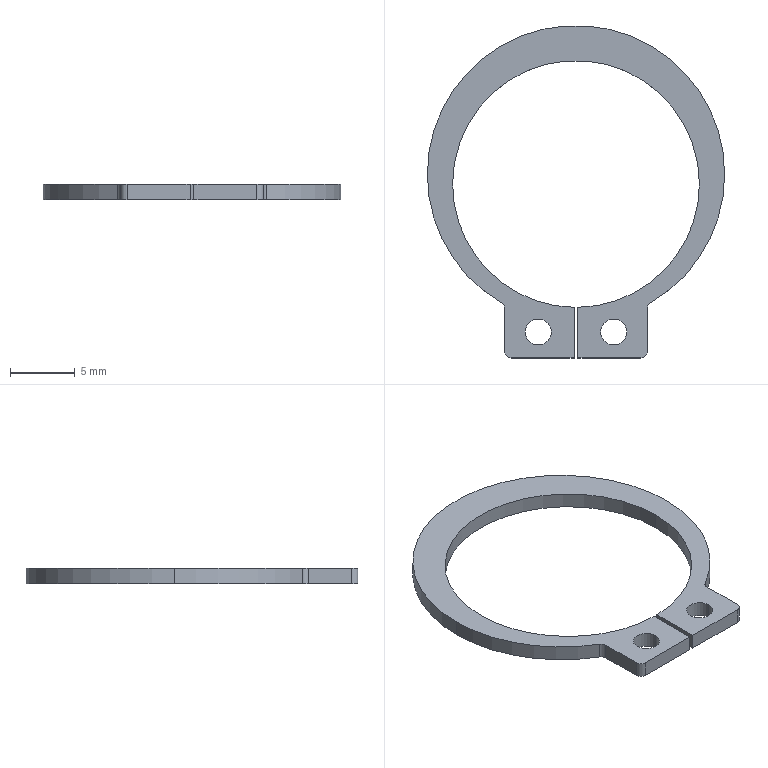Part | SolidWorks | features BaseBody 1 | 1 solid | 22 faces | box 22.9 x 25.6 x 1.2 mm | volume 186.643 mm3 | cylinder 14 | plane 8 | commonest cylinder face diameters 1 x4 2 x4 19 x3 22.9 x3
STEP:
#1=CARTESIAN_POINT('',(-1.9,-11.4,1.2));
#2=VERTEX_POINT('',#1);
#3=CARTESIAN_POINT('',(-3.9,-11.4,1.2));
#4=VERTEX_POINT('',#3);
#5=CARTESIAN_POINT('',(-2.9,-11.4,1.2));
#6=DIRECTION('',(0.,0.,-1.));
#7=DIRECTION('',(-1.,0.,0.));
#8=AXIS2_PLACEMENT_3D('',#5,#6,#7);
#9=CIRCLE('',#8,1.);
#10=EDGE_CURVE('',#2,#4,#9,.T.);
#11=ORIENTED_EDGE('',*,*,#10,.F.);
#12=CARTESIAN_POINT('',(-1.9,-11.4,0.));
#13=VERTEX_POINT('',#12);
#14=CARTESIAN_POINT('',(-1.9,-11.4,1.2));
#15=DIRECTION('',(0.,0.,-1.));
#16=VECTOR('',#15,1000.);
#17=LINE('',#14,#16);
#18=EDGE_CURVE('',#2,#13,#17,.T.);
#19=ORIENTED_EDGE('',*,*,#18,.T.);
#20=CARTESIAN_POINT('',(-3.9,-11.4,0.));
#21=VERTEX_POINT('',#20);
#22=CARTESIAN_POINT('',(-2.9,-11.4,0.));
#23=DIRECTION('',(0.,0.,-1.));
#24=DIRECTION('',(-1.,0.,0.));
#25=AXIS2_PLACEMENT_3D('',#22,#23,#24);
#26=CIRCLE('',#25,1.);
#27=EDGE_CURVE('',#13,#21,#26,.T.);
#28=ORIENTED_EDGE('',*,*,#27,.T.);
#29=CARTESIAN_POINT('',(-3.9,-11.4,1.2));
#30=DIRECTION('',(0.,0.,-1.));
#31=VECTOR('',#30,1000.);
#32=LINE('',#29,#31);
#33=EDGE_CURVE('',#4,#21,#32,.T.);
#34=ORIENTED_EDGE('',*,*,#33,.F.);
#35=EDGE_LOOP('',(#11,#19,#28,#34));
#36=FACE_OUTER_BOUND('',#35,.T.);
#37=CARTESIAN_POINT('',(-2.9,-11.4,1.2));
#38=DIRECTION('',(0.,0.,-1.));
#39=DIRECTION('',(-1.,0.,0.));
#40=AXIS2_PLACEMENT_3D('',#37,#38,#39);
#41=CYLINDRICAL_SURFACE('',#40,1.);
#42=ADVANCED_FACE('',(#36),#41,.F.);
#43=CARTESIAN_POINT('',(3.9,-11.4,1.2));
#44=VERTEX_POINT('',#43);
#45=CARTESIAN_POINT('',(1.9,-11.4,1.2));
#46=VERTEX_POINT('',#45);
#47=CARTESIAN_POINT('',(2.9,-11.4,1.2));
#48=DIRECTION('',(0.,0.,-1.));
#49=DIRECTION('',(-1.,0.,0.));
#50=AXIS2_PLACEMENT_3D('',#47,#48,#49);
#51=CIRCLE('',#50,1.);
#52=EDGE_CURVE('',#44,#46,#51,.T.);
#53=ORIENTED_EDGE('',*,*,#52,.F.);
#54=CARTESIAN_POINT('',(3.9,-11.4,0.));
#55=VERTEX_POINT('',#54);
#56=CARTESIAN_POINT('',(3.9,-11.4,1.2));
#57=DIRECTION('',(0.,0.,-1.));
#58=VECTOR('',#57,1000.);
#59=LINE('',#56,#58);
#60=EDGE_CURVE('',#44,#55,#59,.T.);
#61=ORIENTED_EDGE('',*,*,#60,.T.);
#62=CARTESIAN_POINT('',(1.9,-11.4,0.));
#63=VERTEX_POINT('',#62);
#64=CARTESIAN_POINT('',(2.9,-11.4,0.));
#65=DIRECTION('',(0.,0.,-1.));
#66=DIRECTION('',(-1.,0.,0.));
#67=AXIS2_PLACEMENT_3D('',#64,#65,#66);
#68=CIRCLE('',#67,1.);
#69=EDGE_CURVE('',#55,#63,#68,.T.);
#70=ORIENTED_EDGE('',*,*,#69,.T.);
#71=CARTESIAN_POINT('',(1.9,-11.4,1.2));
#72=DIRECTION('',(0.,0.,-1.));
#73=VECTOR('',#72,1000.);
#74=LINE('',#71,#73);
#75=EDGE_CURVE('',#46,#63,#74,.T.);
#76=ORIENTED_EDGE('',*,*,#75,.F.);
#77=EDGE_LOOP('',(#53,#61,#70,#76));
#78=FACE_OUTER_BOUND('',#77,.T.);
#79=CARTESIAN_POINT('',(2.9,-11.4,1.2));
#80=DIRECTION('',(0.,0.,-1.));
#81=DIRECTION('',(-1.,0.,0.));
#82=AXIS2_PLACEMENT_3D('',#79,#80,#81);
#83=CYLINDRICAL_SURFACE('',#82,1.);
#84=ADVANCED_FACE('',(#78),#83,.F.);
#85=CARTESIAN_POINT('',(9.5,0.,1.2));
#86=VERTEX_POINT('',#85);
#87=CARTESIAN_POINT('',(0.15,-9.499,1.2));
#88=VERTEX_POINT('',#87);
#89=CARTESIAN_POINT('',(0.,0.,1.2));
#90=DIRECTION('',(0.,0.,-1.));
#91=DIRECTION('',(-1.,0.,0.));
#92=AXIS2_PLACEMENT_3D('',#89,#90,#91);
#93=CIRCLE('',#92,9.5);
#94=EDGE_CURVE('',#86,#88,#93,.T.);
#95=ORIENTED_EDGE('',*,*,#94,.F.);
#96=CARTESIAN_POINT('',(9.5,0.,0.));
#97=VERTEX_POINT('',#96);
#98=CARTESIAN_POINT('',(9.5,0.,1.2));
#99=DIRECTION('',(0.,0.,-1.));
#100=VECTOR('',#99,1000.);
#101=LINE('',#98,#100);
#102=EDGE_CURVE('',#86,#97,#101,.T.);
#103=ORIENTED_EDGE('',*,*,#102,.T.);
#104=CARTESIAN_POINT('',(0.15,-9.499,0.));
#105=VERTEX_POINT('',#104);
#106=CARTESIAN_POINT('',(0.,0.,0.));
#107=DIRECTION('',(0.,0.,-1.));
#108=DIRECTION('',(-1.,0.,0.));
#109=AXIS2_PLACEMENT_3D('',#106,#107,#108);
#110=CIRCLE('',#109,9.5);
#111=EDGE_CURVE('',#97,#105,#110,.T.);
#112=ORIENTED_EDGE('',*,*,#111,.T.);
#113=CARTESIAN_POINT('',(0.15,-9.499,1.2));
#114=DIRECTION('',(0.,0.,-1.));
#115=VECTOR('',#114,1000.);
#116=LINE('',#113,#115);
#117=EDGE_CURVE('',#88,#105,#116,.T.);
#118=ORIENTED_EDGE('',*,*,#117,.F.);
#119=EDGE_LOOP('',(#95,#103,#112,#118));
#120=FACE_OUTER_BOUND('',#119,.T.);
#121=CARTESIAN_POINT('',(0.,0.,1.2));
#122=DIRECTION('',(0.,0.,-1.));
#123=DIRECTION('',(-1.,0.,0.));
#124=AXIS2_PLACEMENT_3D('',#121,#122,#123);
#125=CYLINDRICAL_SURFACE('',#124,9.5);
#126=ADVANCED_FACE('',(#120),#125,.F.);
#127=ORIENTED_EDGE('',*,*,#102,.F.);
#128=CARTESIAN_POINT('',(-9.5,0.,1.2));
#129=VERTEX_POINT('',#128);
#130=CARTESIAN_POINT('',(0.,0.,1.2));
#131=DIRECTION('',(0.,0.,-1.));
#132=DIRECTION('',(-1.,0.,0.));
#133=AXIS2_PLACEMENT_3D('',#130,#131,#132);
#134=CIRCLE('',#133,9.5);
#135=EDGE_CURVE('',#129,#86,#134,.T.);
#136=ORIENTED_EDGE('',*,*,#135,.F.);
#137=CARTESIAN_POINT('',(-9.5,0.,0.));
#138=VERTEX_POINT('',#137);
#139=CARTESIAN_POINT('',(-9.5,0.,1.2));
#140=DIRECTION('',(0.,0.,-1.));
#141=VECTOR('',#140,1000.);
#142=LINE('',#139,#141);
#143=EDGE_CURVE('',#129,#138,#142,.T.);
#144=ORIENTED_EDGE('',*,*,#143,.T.);
#145=CARTESIAN_POINT('',(0.,0.,0.));
#146=DIRECTION('',(0.,0.,-1.));
#147=DIRECTION('',(-1.,0.,0.));
#148=AXIS2_PLACEMENT_3D('',#145,#146,#147);
#149=CIRCLE('',#148,9.5);
#150=EDGE_CURVE('',#138,#97,#149,.T.);
#151=ORIENTED_EDGE('',*,*,#150,.T.);
#152=EDGE_LOOP('',(#127,#136,#144,#151));
#153=FACE_OUTER_BOUND('',#152,.T.);
#154=CARTESIAN_POINT('',(0.,0.,1.2));
#155=DIRECTION('',(0.,0.,-1.));
#156=DIRECTION('',(-1.,0.,0.));
#157=AXIS2_PLACEMENT_3D('',#154,#155,#156);
#158=CYLINDRICAL_SURFACE('',#157,9.5);
#159=ADVANCED_FACE('',(#153),#158,.F.);
#160=CARTESIAN_POINT('',(11.45,0.75,1.2));
#161=VERTEX_POINT('',#160);
#162=CARTESIAN_POINT('',(-11.45,0.75,1.2));
#163=VERTEX_POINT('',#162);
#164=CARTESIAN_POINT('',(0.,0.75,1.2));
#165=DIRECTION('',(0.,0.,1.));
#166=DIRECTION('',(1.,0.,0.));
#167=AXIS2_PLACEMENT_3D('',#164,#165,#166);
#168=CIRCLE('',#167,11.45);
#169=EDGE_CURVE('',#161,#163,#168,.T.);
#170=ORIENTED_EDGE('',*,*,#169,.F.);
#171=CARTESIAN_POINT('',(11.45,0.75,0.));
#172=VERTEX_POINT('',#171);
#173=CARTESIAN_POINT('',(11.45,0.75,1.2));
#174=DIRECTION('',(0.,0.,-1.));
#175=VECTOR('',#174,1000.);
#176=LINE('',#173,#175);
#177=EDGE_CURVE('',#161,#172,#176,.T.);
#178=ORIENTED_EDGE('',*,*,#177,.T.);
#179=CARTESIAN_POINT('',(-11.45,0.75,0.));
#180=VERTEX_POINT('',#179);
#181=CARTESIAN_POINT('',(0.,0.75,0.));
#182=DIRECTION('',(0.,0.,1.));
#183=DIRECTION('',(1.,0.,0.));
#184=AXIS2_PLACEMENT_3D('',#181,#182,#183);
#185=CIRCLE('',#184,11.45);
#186=EDGE_CURVE('',#172,#180,#185,.T.);
#187=ORIENTED_EDGE('',*,*,#186,.T.);
#188=CARTESIAN_POINT('',(-11.45,0.75,1.2));
#189=DIRECTION('',(0.,0.,-1.));
#190=VECTOR('',#189,1000.);
#191=LINE('',#188,#190);
#192=EDGE_CURVE('',#163,#180,#191,.T.);
#193=ORIENTED_EDGE('',*,*,#192,.F.);
#194=EDGE_LOOP('',(#170,#178,#187,#193));
#195=FACE_OUTER_BOUND('',#194,.T.);
#196=CARTESIAN_POINT('',(0.,0.75,1.2));
#197=DIRECTION('',(0.,0.,-1.));
#198=DIRECTION('',(-1.,0.,0.));
#199=AXIS2_PLACEMENT_3D('',#196,#197,#198);
#200=CYLINDRICAL_SURFACE('',#199,11.45);
#201=ADVANCED_FACE('',(#195),#200,.T.);
#202=CARTESIAN_POINT('',(-5.749,-9.152,1.2));
#203=VERTEX_POINT('',#202);
#204=CARTESIAN_POINT('',(0.,0.75,1.2));
#205=DIRECTION('',(0.,0.,1.));
#206=DIRECTION('',(1.,0.,0.));
#207=AXIS2_PLACEMENT_3D('',#204,#205,#206);
#208=CIRCLE('',#207,11.45);
#209=EDGE_CURVE('',#163,#203,#208,.T.);
#210=ORIENTED_EDGE('',*,*,#209,.F.);
#211=ORIENTED_EDGE('',*,*,#192,.T.);
#212=CARTESIAN_POINT('',(-5.749,-9.152,0.));
#213=VERTEX_POINT('',#212);
#214=CARTESIAN_POINT('',(0.,0.75,0.));
#215=DIRECTION('',(0.,0.,1.));
#216=DIRECTION('',(1.,0.,0.));
#217=AXIS2_PLACEMENT_3D('',#214,#215,#216);
#218=CIRCLE('',#217,11.45);
#219=EDGE_CURVE('',#180,#213,#218,.T.);
#220=ORIENTED_EDGE('',*,*,#219,.T.);
#221=CARTESIAN_POINT('',(-5.749,-9.152,1.2));
#222=DIRECTION('',(0.,0.,-1.));
#223=VECTOR('',#222,1000.);
#224=LINE('',#221,#223);
#225=EDGE_CURVE('',#203,#213,#224,.T.);
#226=ORIENTED_EDGE('',*,*,#225,.F.);
#227=EDGE_LOOP('',(#210,#211,#220,#226));
#228=FACE_OUTER_BOUND('',#227,.T.);
#229=CARTESIAN_POINT('',(0.,0.75,1.2));
#230=DIRECTION('',(0.,0.,-1.));
#231=DIRECTION('',(-1.,0.,0.));
#232=AXIS2_PLACEMENT_3D('',#229,#230,#231);
#233=CYLINDRICAL_SURFACE('',#232,11.45);
#234=ADVANCED_FACE('',(#228),#233,.T.);
#235=CARTESIAN_POINT('',(2.9,-11.4,0.));
#236=DIRECTION('',(0.,0.,-1.));
#237=DIRECTION('',(-1.,0.,0.));
#238=AXIS2_PLACEMENT_3D('',#235,#236,#237);
#239=CIRCLE('',#238,1.);
#240=EDGE_CURVE('',#63,#55,#239,.T.);
#241=ORIENTED_EDGE('',*,*,#240,.F.);
#242=ORIENTED_EDGE('',*,*,#69,.F.);
#243=EDGE_LOOP('',(#241,#242));
#244=FACE_BOUND('',#243,.T.);
#245=CARTESIAN_POINT('',(-2.9,-11.4,0.));
#246=DIRECTION('',(0.,0.,-1.));
#247=DIRECTION('',(-1.,0.,0.));
#248=AXIS2_PLACEMENT_3D('',#245,#246,#247);
#249=CIRCLE('',#248,1.);
#250=EDGE_CURVE('',#21,#13,#249,.T.);
#251=ORIENTED_EDGE('',*,*,#250,.F.);
#252=ORIENTED_EDGE('',*,*,#27,.F.);
#253=EDGE_LOOP('',(#251,#252));
#254=FACE_BOUND('',#253,.T.);
#255=CARTESIAN_POINT('',(5.5,-9.585,0.));
#256=VERTEX_POINT('',#255);
#257=CARTESIAN_POINT('',(5.749,-9.152,0.));
#258=VERTEX_POINT('',#257);
#259=CARTESIAN_POINT('',(6.,-9.585,0.));
#260=DIRECTION('',(0.,0.,-1.));
#261=DIRECTION('',(-1.,0.,0.));
#262=AXIS2_PLACEMENT_3D('',#259,#260,#261);
#263=CIRCLE('',#262,0.5);
#264=EDGE_CURVE('',#256,#258,#263,.T.);
#265=ORIENTED_EDGE('',*,*,#264,.F.);
#266=CARTESIAN_POINT('',(5.5,-12.9,0.));
#267=VERTEX_POINT('',#266);
#268=CARTESIAN_POINT('',(5.5,-12.9,0.));
#269=DIRECTION('',(0.,1.,0.));
#270=VECTOR('',#269,1000.);
#271=LINE('',#268,#270);
#272=EDGE_CURVE('',#267,#256,#271,.T.);
#273=ORIENTED_EDGE('',*,*,#272,.F.);
#274=CARTESIAN_POINT('',(5.,-13.4,0.));
#275=VERTEX_POINT('',#274);
#276=CARTESIAN_POINT('',(5.,-12.9,0.));
#277=DIRECTION('',(0.,0.,1.));
#278=DIRECTION('',(1.,0.,0.));
#279=AXIS2_PLACEMENT_3D('',#276,#277,#278);
#280=CIRCLE('',#279,0.5);
#281=EDGE_CURVE('',#275,#267,#280,.T.);
#282=ORIENTED_EDGE('',*,*,#281,.F.);
#283=CARTESIAN_POINT('',(0.15,-13.4,0.));
#284=VERTEX_POINT('',#283);
#285=CARTESIAN_POINT('',(0.15,-13.4,0.));
#286=DIRECTION('',(1.,0.,0.));
#287=VECTOR('',#286,1000.);
#288=LINE('',#285,#287);
#289=EDGE_CURVE('',#284,#275,#288,.T.);
#290=ORIENTED_EDGE('',*,*,#289,.F.);
#291=CARTESIAN_POINT('',(0.15,-9.499,0.));
#292=DIRECTION('',(0.,-1.,0.));
#293=VECTOR('',#292,1000.);
#294=LINE('',#291,#293);
#295=EDGE_CURVE('',#105,#284,#294,.T.);
#296=ORIENTED_EDGE('',*,*,#295,.F.);
#297=ORIENTED_EDGE('',*,*,#111,.F.);
#298=ORIENTED_EDGE('',*,*,#150,.F.);
#299=CARTESIAN_POINT('',(-0.15,-9.499,0.));
#300=VERTEX_POINT('',#299);
#301=CARTESIAN_POINT('',(0.,0.,0.));
#302=DIRECTION('',(0.,0.,-1.));
#303=DIRECTION('',(-1.,0.,0.));
#304=AXIS2_PLACEMENT_3D('',#301,#302,#303);
#305=CIRCLE('',#304,9.5);
#306=EDGE_CURVE('',#300,#138,#305,.T.);
#307=ORIENTED_EDGE('',*,*,#306,.F.);
#308=CARTESIAN_POINT('',(-0.15,-13.4,0.));
#309=VERTEX_POINT('',#308);
#310=CARTESIAN_POINT('',(-0.15,-13.4,0.));
#311=DIRECTION('',(0.,1.,0.));
#312=VECTOR('',#311,1000.);
#313=LINE('',#310,#312);
#314=EDGE_CURVE('',#309,#300,#313,.T.);
#315=ORIENTED_EDGE('',*,*,#314,.F.);
#316=CARTESIAN_POINT('',(-5.,-13.4,0.));
#317=VERTEX_POINT('',#316);
#318=CARTESIAN_POINT('',(-5.,-13.4,0.));
#319=DIRECTION('',(1.,0.,0.));
#320=VECTOR('',#319,1000.);
#321=LINE('',#318,#320);
#322=EDGE_CURVE('',#317,#309,#321,.T.);
#323=ORIENTED_EDGE('',*,*,#322,.F.);
#324=CARTESIAN_POINT('',(-5.5,-12.9,0.));
#325=VERTEX_POINT('',#324);
#326=CARTESIAN_POINT('',(-5.,-12.9,0.));
#327=DIRECTION('',(0.,0.,1.));
#328=DIRECTION('',(1.,0.,0.));
#329=AXIS2_PLACEMENT_3D('',#326,#327,#328);
#330=CIRCLE('',#329,0.5);
#331=EDGE_CURVE('',#325,#317,#330,.T.);
#332=ORIENTED_EDGE('',*,*,#331,.F.);
#333=CARTESIAN_POINT('',(-5.5,-9.585,0.));
#334=VERTEX_POINT('',#333);
#335=CARTESIAN_POINT('',(-5.5,-9.585,0.));
#336=DIRECTION('',(0.,-1.,0.));
#337=VECTOR('',#336,1000.);
#338=LINE('',#335,#337);
#339=EDGE_CURVE('',#334,#325,#338,.T.);
#340=ORIENTED_EDGE('',*,*,#339,.F.);
#341=CARTESIAN_POINT('',(-6.,-9.585,0.));
#342=DIRECTION('',(0.,0.,-1.));
#343=DIRECTION('',(-1.,0.,0.));
#344=AXIS2_PLACEMENT_3D('',#341,#342,#343);
#345=CIRCLE('',#344,0.5);
#346=EDGE_CURVE('',#213,#334,#345,.T.);
#347=ORIENTED_EDGE('',*,*,#346,.F.);
#348=ORIENTED_EDGE('',*,*,#219,.F.);
#349=ORIENTED_EDGE('',*,*,#186,.F.);
#350=CARTESIAN_POINT('',(0.,0.75,0.));
#351=DIRECTION('',(0.,0.,1.));
#352=DIRECTION('',(1.,0.,0.));
#353=AXIS2_PLACEMENT_3D('',#350,#351,#352);
#354=CIRCLE('',#353,11.45);
#355=EDGE_CURVE('',#258,#172,#354,.T.);
#356=ORIENTED_EDGE('',*,*,#355,.F.);
#357=EDGE_LOOP('',(#265,#273,#282,#290,#296,#297,#298,#307,#315,#323,#332,#340,#347,#348,#349,#356));
#358=FACE_OUTER_BOUND('',#357,.T.);
#359=CARTESIAN_POINT('',(6.,-9.585,0.));
#360=DIRECTION('',(0.,0.,-1.));
#361=DIRECTION('',(0.,-1.,0.));
#362=AXIS2_PLACEMENT_3D('',#359,#360,#361);
#363=PLANE('',#362);
#364=ADVANCED_FACE('',(#244,#254,#358),#363,.T.);
#365=CARTESIAN_POINT('',(2.9,-11.4,1.2));
#366=DIRECTION('',(0.,0.,-1.));
#367=DIRECTION('',(-1.,0.,0.));
#368=AXIS2_PLACEMENT_3D('',#365,#366,#367);
#369=CIRCLE('',#368,1.);
#370=EDGE_CURVE('',#46,#44,#369,.T.);
#371=ORIENTED_EDGE('',*,*,#370,.T.);
#372=ORIENTED_EDGE('',*,*,#52,.T.);
#373=EDGE_LOOP('',(#371,#372));
#374=FACE_BOUND('',#373,.T.);
#375=CARTESIAN_POINT('',(-2.9,-11.4,1.2));
#376=DIRECTION('',(0.,0.,-1.));
#377=DIRECTION('',(-1.,0.,0.));
#378=AXIS2_PLACEMENT_3D('',#375,#376,#377);
#379=CIRCLE('',#378,1.);
#380=EDGE_CURVE('',#4,#2,#379,.T.);
#381=ORIENTED_EDGE('',*,*,#380,.T.);
#382=ORIENTED_EDGE('',*,*,#10,.T.);
#383=EDGE_LOOP('',(#381,#382));
#384=FACE_BOUND('',#383,.T.);
#385=CARTESIAN_POINT('',(5.5,-9.585,1.2));
#386=VERTEX_POINT('',#385);
#387=CARTESIAN_POINT('',(5.749,-9.152,1.2));
#388=VERTEX_POINT('',#387);
#389=CARTESIAN_POINT('',(6.,-9.585,1.2));
#390=DIRECTION('',(0.,0.,-1.));
#391=DIRECTION('',(-1.,0.,0.));
#392=AXIS2_PLACEMENT_3D('',#389,#390,#391);
#393=CIRCLE('',#392,0.5);
#394=EDGE_CURVE('',#386,#388,#393,.T.);
#395=ORIENTED_EDGE('',*,*,#394,.T.);
#396=CARTESIAN_POINT('',(0.,0.75,1.2));
#397=DIRECTION('',(0.,0.,1.));
#398=DIRECTION('',(1.,0.,0.));
#399=AXIS2_PLACEMENT_3D('',#396,#397,#398);
#400=CIRCLE('',#399,11.45);
#401=EDGE_CURVE('',#388,#161,#400,.T.);
#402=ORIENTED_EDGE('',*,*,#401,.T.);
#403=ORIENTED_EDGE('',*,*,#169,.T.);
#404=ORIENTED_EDGE('',*,*,#209,.T.);
#405=CARTESIAN_POINT('',(-5.5,-9.585,1.2));
#406=VERTEX_POINT('',#405);
#407=CARTESIAN_POINT('',(-6.,-9.585,1.2));
#408=DIRECTION('',(0.,0.,-1.));
#409=DIRECTION('',(-1.,0.,0.));
#410=AXIS2_PLACEMENT_3D('',#407,#408,#409);
#411=CIRCLE('',#410,0.5);
#412=EDGE_CURVE('',#203,#406,#411,.T.);
#413=ORIENTED_EDGE('',*,*,#412,.T.);
#414=CARTESIAN_POINT('',(-5.5,-12.9,1.2));
#415=VERTEX_POINT('',#414);
#416=CARTESIAN_POINT('',(-5.5,-9.585,1.2));
#417=DIRECTION('',(0.,-1.,0.));
#418=VECTOR('',#417,1000.);
#419=LINE('',#416,#418);
#420=EDGE_CURVE('',#406,#415,#419,.T.);
#421=ORIENTED_EDGE('',*,*,#420,.T.);
#422=CARTESIAN_POINT('',(-5.,-13.4,1.2));
#423=VERTEX_POINT('',#422);
#424=CARTESIAN_POINT('',(-5.,-12.9,1.2));
#425=DIRECTION('',(0.,0.,1.));
#426=DIRECTION('',(1.,0.,0.));
#427=AXIS2_PLACEMENT_3D('',#424,#425,#426);
#428=CIRCLE('',#427,0.5);
#429=EDGE_CURVE('',#415,#423,#428,.T.);
#430=ORIENTED_EDGE('',*,*,#429,.T.);
#431=CARTESIAN_POINT('',(-0.15,-13.4,1.2));
#432=VERTEX_POINT('',#431);
#433=CARTESIAN_POINT('',(-5.,-13.4,1.2));
#434=DIRECTION('',(1.,0.,0.));
#435=VECTOR('',#434,1000.);
#436=LINE('',#433,#435);
#437=EDGE_CURVE('',#423,#432,#436,.T.);
#438=ORIENTED_EDGE('',*,*,#437,.T.);
#439=CARTESIAN_POINT('',(-0.15,-9.499,1.2));
#440=VERTEX_POINT('',#439);
#441=CARTESIAN_POINT('',(-0.15,-13.4,1.2));
#442=DIRECTION('',(0.,1.,0.));
#443=VECTOR('',#442,1000.);
#444=LINE('',#441,#443);
#445=EDGE_CURVE('',#432,#440,#444,.T.);
#446=ORIENTED_EDGE('',*,*,#445,.T.);
#447=CARTESIAN_POINT('',(0.,0.,1.2));
#448=DIRECTION('',(0.,0.,-1.));
#449=DIRECTION('',(-1.,0.,0.));
#450=AXIS2_PLACEMENT_3D('',#447,#448,#449);
#451=CIRCLE('',#450,9.5);
#452=EDGE_CURVE('',#440,#129,#451,.T.);
#453=ORIENTED_EDGE('',*,*,#452,.T.);
#454=ORIENTED_EDGE('',*,*,#135,.T.);
#455=ORIENTED_EDGE('',*,*,#94,.T.);
#456=CARTESIAN_POINT('',(0.15,-13.4,1.2));
#457=VERTEX_POINT('',#456);
#458=CARTESIAN_POINT('',(0.15,-9.499,1.2));
#459=DIRECTION('',(0.,-1.,0.));
#460=VECTOR('',#459,1000.);
#461=LINE('',#458,#460);
#462=EDGE_CURVE('',#88,#457,#461,.T.);
#463=ORIENTED_EDGE('',*,*,#462,.T.);
#464=CARTESIAN_POINT('',(5.,-13.4,1.2));
#465=VERTEX_POINT('',#464);
#466=CARTESIAN_POINT('',(0.15,-13.4,1.2));
#467=DIRECTION('',(1.,0.,0.));
#468=VECTOR('',#467,1000.);
#469=LINE('',#466,#468);
#470=EDGE_CURVE('',#457,#465,#469,.T.);
#471=ORIENTED_EDGE('',*,*,#470,.T.);
#472=CARTESIAN_POINT('',(5.5,-12.9,1.2));
#473=VERTEX_POINT('',#472);
#474=CARTESIAN_POINT('',(5.,-12.9,1.2));
#475=DIRECTION('',(0.,0.,1.));
#476=DIRECTION('',(1.,0.,0.));
#477=AXIS2_PLACEMENT_3D('',#474,#475,#476);
#478=CIRCLE('',#477,0.5);
#479=EDGE_CURVE('',#465,#473,#478,.T.);
#480=ORIENTED_EDGE('',*,*,#479,.T.);
#481=CARTESIAN_POINT('',(5.5,-12.9,1.2));
#482=DIRECTION('',(0.,1.,0.));
#483=VECTOR('',#482,1000.);
#484=LINE('',#481,#483);
#485=EDGE_CURVE('',#473,#386,#484,.T.);
#486=ORIENTED_EDGE('',*,*,#485,.T.);
#487=EDGE_LOOP('',(#395,#402,#403,#404,#413,#421,#430,#438,#446,#453,#454,#455,#463,#471,#480,#486));
#488=FACE_OUTER_BOUND('',#487,.T.);
#489=CARTESIAN_POINT('',(6.,-9.585,1.2));
#490=DIRECTION('',(0.,0.,-1.));
#491=DIRECTION('',(0.,-1.,0.));
#492=AXIS2_PLACEMENT_3D('',#489,#490,#491);
#493=PLANE('',#492);
#494=ADVANCED_FACE('',(#374,#384,#488),#493,.F.);
#495=ORIENTED_EDGE('',*,*,#272,.T.);
#496=CARTESIAN_POINT('',(5.5,-9.585,1.2));
#497=DIRECTION('',(0.,0.,-1.));
#498=VECTOR('',#497,1000.);
#499=LINE('',#496,#498);
#500=EDGE_CURVE('',#386,#256,#499,.T.);
#501=ORIENTED_EDGE('',*,*,#500,.F.);
#502=ORIENTED_EDGE('',*,*,#485,.F.);
#503=CARTESIAN_POINT('',(5.5,-12.9,1.2));
#504=DIRECTION('',(0.,0.,-1.));
#505=VECTOR('',#504,1000.);
#506=LINE('',#503,#505);
#507=EDGE_CURVE('',#473,#267,#506,.T.);
#508=ORIENTED_EDGE('',*,*,#507,.T.);
#509=EDGE_LOOP('',(#495,#501,#502,#508));
#510=FACE_OUTER_BOUND('',#509,.T.);
#511=CARTESIAN_POINT('',(5.5,-12.9,1.2));
#512=DIRECTION('',(-1.,0.,0.));
#513=DIRECTION('',(0.,0.,1.));
#514=AXIS2_PLACEMENT_3D('',#511,#512,#513);
#515=PLANE('',#514);
#516=ADVANCED_FACE('',(#510),#515,.F.);
#517=ORIENTED_EDGE('',*,*,#281,.T.);
#518=ORIENTED_EDGE('',*,*,#507,.F.);
#519=ORIENTED_EDGE('',*,*,#479,.F.);
#520=CARTESIAN_POINT('',(5.,-13.4,1.2));
#521=DIRECTION('',(0.,0.,-1.));
#522=VECTOR('',#521,1000.);
#523=LINE('',#520,#522);
#524=EDGE_CURVE('',#465,#275,#523,.T.);
#525=ORIENTED_EDGE('',*,*,#524,.T.);
#526=EDGE_LOOP('',(#517,#518,#519,#525));
#527=FACE_OUTER_BOUND('',#526,.T.);
#528=CARTESIAN_POINT('',(5.,-12.9,1.2));
#529=DIRECTION('',(0.,0.,-1.));
#530=DIRECTION('',(-1.,0.,0.));
#531=AXIS2_PLACEMENT_3D('',#528,#529,#530);
#532=CYLINDRICAL_SURFACE('',#531,0.5);
#533=ADVANCED_FACE('',(#527),#532,.T.);
#534=ORIENTED_EDGE('',*,*,#289,.T.);
#535=ORIENTED_EDGE('',*,*,#524,.F.);
#536=ORIENTED_EDGE('',*,*,#470,.F.);
#537=CARTESIAN_POINT('',(0.15,-13.4,1.2));
#538=DIRECTION('',(0.,0.,-1.));
#539=VECTOR('',#538,1000.);
#540=LINE('',#537,#539);
#541=EDGE_CURVE('',#457,#284,#540,.T.);
#542=ORIENTED_EDGE('',*,*,#541,.T.);
#543=EDGE_LOOP('',(#534,#535,#536,#542));
#544=FACE_OUTER_BOUND('',#543,.T.);
#545=CARTESIAN_POINT('',(0.15,-13.4,1.2));
#546=DIRECTION('',(0.,1.,0.));
#547=DIRECTION('',(1.,0.,0.));
#548=AXIS2_PLACEMENT_3D('',#545,#546,#547);
#549=PLANE('',#548);
#550=ADVANCED_FACE('',(#544),#549,.F.);
#551=ORIENTED_EDGE('',*,*,#295,.T.);
#552=ORIENTED_EDGE('',*,*,#541,.F.);
#553=ORIENTED_EDGE('',*,*,#462,.F.);
#554=ORIENTED_EDGE('',*,*,#117,.T.);
#555=EDGE_LOOP('',(#551,#552,#553,#554));
#556=FACE_OUTER_BOUND('',#555,.T.);
#557=CARTESIAN_POINT('',(0.15,-9.499,1.2));
#558=DIRECTION('',(1.,0.,0.));
#559=DIRECTION('',(0.,1.,0.));
#560=AXIS2_PLACEMENT_3D('',#557,#558,#559);
#561=PLANE('',#560);
#562=ADVANCED_FACE('',(#556),#561,.F.);
#563=ORIENTED_EDGE('',*,*,#314,.T.);
#564=CARTESIAN_POINT('',(-0.15,-9.499,1.2));
#565=DIRECTION('',(0.,0.,-1.));
#566=VECTOR('',#565,1000.);
#567=LINE('',#564,#566);
#568=EDGE_CURVE('',#440,#300,#567,.T.);
#569=ORIENTED_EDGE('',*,*,#568,.F.);
#570=ORIENTED_EDGE('',*,*,#445,.F.);
#571=CARTESIAN_POINT('',(-0.15,-13.4,1.2));
#572=DIRECTION('',(0.,0.,-1.));
#573=VECTOR('',#572,1000.);
#574=LINE('',#571,#573);
#575=EDGE_CURVE('',#432,#309,#574,.T.);
#576=ORIENTED_EDGE('',*,*,#575,.T.);
#577=EDGE_LOOP('',(#563,#569,#570,#576));
#578=FACE_OUTER_BOUND('',#577,.T.);
#579=CARTESIAN_POINT('',(-0.15,-13.4,1.2));
#580=DIRECTION('',(-1.,0.,0.));
#581=DIRECTION('',(0.,0.,1.));
#582=AXIS2_PLACEMENT_3D('',#579,#580,#581);
#583=PLANE('',#582);
#584=ADVANCED_FACE('',(#578),#583,.F.);
#585=ORIENTED_EDGE('',*,*,#322,.T.);
#586=ORIENTED_EDGE('',*,*,#575,.F.);
#587=ORIENTED_EDGE('',*,*,#437,.F.);
#588=CARTESIAN_POINT('',(-5.,-13.4,1.2));
#589=DIRECTION('',(0.,0.,-1.));
#590=VECTOR('',#589,1000.);
#591=LINE('',#588,#590);
#592=EDGE_CURVE('',#423,#317,#591,.T.);
#593=ORIENTED_EDGE('',*,*,#592,.T.);
#594=EDGE_LOOP('',(#585,#586,#587,#593));
#595=FACE_OUTER_BOUND('',#594,.T.);
#596=CARTESIAN_POINT('',(-5.,-13.4,1.2));
#597=DIRECTION('',(0.,1.,0.));
#598=DIRECTION('',(1.,0.,0.));
#599=AXIS2_PLACEMENT_3D('',#596,#597,#598);
#600=PLANE('',#599);
#601=ADVANCED_FACE('',(#595),#600,.F.);
#602=ORIENTED_EDGE('',*,*,#331,.T.);
#603=ORIENTED_EDGE('',*,*,#592,.F.);
#604=ORIENTED_EDGE('',*,*,#429,.F.);
#605=CARTESIAN_POINT('',(-5.5,-12.9,1.2));
#606=DIRECTION('',(0.,0.,-1.));
#607=VECTOR('',#606,1000.);
#608=LINE('',#605,#607);
#609=EDGE_CURVE('',#415,#325,#608,.T.);
#610=ORIENTED_EDGE('',*,*,#609,.T.);
#611=EDGE_LOOP('',(#602,#603,#604,#610));
#612=FACE_OUTER_BOUND('',#611,.T.);
#613=CARTESIAN_POINT('',(-5.,-12.9,1.2));
#614=DIRECTION('',(0.,0.,-1.));
#615=DIRECTION('',(-1.,0.,0.));
#616=AXIS2_PLACEMENT_3D('',#613,#614,#615);
#617=CYLINDRICAL_SURFACE('',#616,0.5);
#618=ADVANCED_FACE('',(#612),#617,.T.);
#619=ORIENTED_EDGE('',*,*,#339,.T.);
#620=ORIENTED_EDGE('',*,*,#609,.F.);
#621=ORIENTED_EDGE('',*,*,#420,.F.);
#622=CARTESIAN_POINT('',(-5.5,-9.585,1.2));
#623=DIRECTION('',(0.,0.,-1.));
#624=VECTOR('',#623,1000.);
#625=LINE('',#622,#624);
#626=EDGE_CURVE('',#406,#334,#625,.T.);
#627=ORIENTED_EDGE('',*,*,#626,.T.);
#628=EDGE_LOOP('',(#619,#620,#621,#627));
#629=FACE_OUTER_BOUND('',#628,.T.);
#630=CARTESIAN_POINT('',(-5.5,-9.585,1.2));
#631=DIRECTION('',(1.,0.,0.));
#632=DIRECTION('',(0.,1.,0.));
#633=AXIS2_PLACEMENT_3D('',#630,#631,#632);
#634=PLANE('',#633);
#635=ADVANCED_FACE('',(#629),#634,.F.);
#636=ORIENTED_EDGE('',*,*,#346,.T.);
#637=ORIENTED_EDGE('',*,*,#626,.F.);
#638=ORIENTED_EDGE('',*,*,#412,.F.);
#639=ORIENTED_EDGE('',*,*,#225,.T.);
#640=EDGE_LOOP('',(#636,#637,#638,#639));
#641=FACE_OUTER_BOUND('',#640,.T.);
#642=CARTESIAN_POINT('',(-6.,-9.585,1.2));
#643=DIRECTION('',(0.,0.,-1.));
#644=DIRECTION('',(-1.,0.,0.));
#645=AXIS2_PLACEMENT_3D('',#642,#643,#644);
#646=CYLINDRICAL_SURFACE('',#645,0.5);
#647=ADVANCED_FACE('',(#641),#646,.F.);
#648=ORIENTED_EDGE('',*,*,#264,.T.);
#649=CARTESIAN_POINT('',(5.749,-9.152,1.2));
#650=DIRECTION('',(0.,0.,-1.));
#651=VECTOR('',#650,1000.);
#652=LINE('',#649,#651);
#653=EDGE_CURVE('',#388,#258,#652,.T.);
#654=ORIENTED_EDGE('',*,*,#653,.F.);
#655=ORIENTED_EDGE('',*,*,#394,.F.);
#656=ORIENTED_EDGE('',*,*,#500,.T.);
#657=EDGE_LOOP('',(#648,#654,#655,#656));
#658=FACE_OUTER_BOUND('',#657,.T.);
#659=CARTESIAN_POINT('',(6.,-9.585,1.2));
#660=DIRECTION('',(0.,0.,-1.));
#661=DIRECTION('',(-1.,0.,0.));
#662=AXIS2_PLACEMENT_3D('',#659,#660,#661);
#663=CYLINDRICAL_SURFACE('',#662,0.5);
#664=ADVANCED_FACE('',(#658),#663,.F.);
#665=ORIENTED_EDGE('',*,*,#177,.F.);
#666=ORIENTED_EDGE('',*,*,#401,.F.);
#667=ORIENTED_EDGE('',*,*,#653,.T.);
#668=ORIENTED_EDGE('',*,*,#355,.T.);
#669=EDGE_LOOP('',(#665,#666,#667,#668));
#670=FACE_OUTER_BOUND('',#669,.T.);
#671=CARTESIAN_POINT('',(0.,0.75,1.2));
#672=DIRECTION('',(0.,0.,-1.));
#673=DIRECTION('',(-1.,0.,0.));
#674=AXIS2_PLACEMENT_3D('',#671,#672,#673);
#675=CYLINDRICAL_SURFACE('',#674,11.45);
#676=ADVANCED_FACE('',(#670),#675,.T.);
#677=ORIENTED_EDGE('',*,*,#143,.F.);
#678=ORIENTED_EDGE('',*,*,#452,.F.);
#679=ORIENTED_EDGE('',*,*,#568,.T.);
#680=ORIENTED_EDGE('',*,*,#306,.T.);
#681=EDGE_LOOP('',(#677,#678,#679,#680));
#682=FACE_OUTER_BOUND('',#681,.T.);
#683=CARTESIAN_POINT('',(0.,0.,1.2));
#684=DIRECTION('',(0.,0.,-1.));
#685=DIRECTION('',(-1.,0.,0.));
#686=AXIS2_PLACEMENT_3D('',#683,#684,#685);
#687=CYLINDRICAL_SURFACE('',#686,9.5);
#688=ADVANCED_FACE('',(#682),#687,.F.);
#689=ORIENTED_EDGE('',*,*,#60,.F.);
#690=ORIENTED_EDGE('',*,*,#370,.F.);
#691=ORIENTED_EDGE('',*,*,#75,.T.);
#692=ORIENTED_EDGE('',*,*,#240,.T.);
#693=EDGE_LOOP('',(#689,#690,#691,#692));
#694=FACE_OUTER_BOUND('',#693,.T.);
#695=CARTESIAN_POINT('',(2.9,-11.4,1.2));
#696=DIRECTION('',(0.,0.,-1.));
#697=DIRECTION('',(-1.,0.,0.));
#698=AXIS2_PLACEMENT_3D('',#695,#696,#697);
#699=CYLINDRICAL_SURFACE('',#698,1.);
#700=ADVANCED_FACE('',(#694),#699,.F.);
#701=ORIENTED_EDGE('',*,*,#18,.F.);
#702=ORIENTED_EDGE('',*,*,#380,.F.);
#703=ORIENTED_EDGE('',*,*,#33,.T.);
#704=ORIENTED_EDGE('',*,*,#250,.T.);
#705=EDGE_LOOP('',(#701,#702,#703,#704));
#706=FACE_OUTER_BOUND('',#705,.T.);
#707=CARTESIAN_POINT('',(-2.9,-11.4,1.2));
#708=DIRECTION('',(0.,0.,-1.));
#709=DIRECTION('',(-1.,0.,0.));
#710=AXIS2_PLACEMENT_3D('',#707,#708,#709);
#711=CYLINDRICAL_SURFACE('',#710,1.);
#712=ADVANCED_FACE('',(#706),#711,.F.);
#713=CLOSED_SHELL('',(#42,#84,#126,#159,#201,#234,#364,#494,#516,#533,#550,#562,#584,#601,#618,#635,#647,#664,#676,#688,#700,#712));
#714=MANIFOLD_SOLID_BREP('',#713);
#715=CARTESIAN_POINT('',(0.,0.,0.));
#716=DIRECTION('',(0.,0.,1.));
#717=DIRECTION('',(1.,0.,0.));
#718=AXIS2_PLACEMENT_3D('',#715,#716,#717);
#719=(LENGTH_UNIT()NAMED_UNIT(*)SI_UNIT(.MILLI.,.METRE.));
#720=UNCERTAINTY_MEASURE_WITH_UNIT(LENGTH_MEASURE(0.00001),#719,'','');
#721=(NAMED_UNIT(*)PLANE_ANGLE_UNIT()SI_UNIT($,.RADIAN.));
#722=(NAMED_UNIT(*)SI_UNIT($,.STERADIAN.)SOLID_ANGLE_UNIT());
#723=(GEOMETRIC_REPRESENTATION_CONTEXT(3)GLOBAL_UNCERTAINTY_ASSIGNED_CONTEXT((#720))GLOBAL_UNIT_ASSIGNED_CONTEXT((#719,#721,#722))REPRESENTATION_CONTEXT('',''));
#724=ADVANCED_BREP_SHAPE_REPRESENTATION('',(#714,#718),#723);